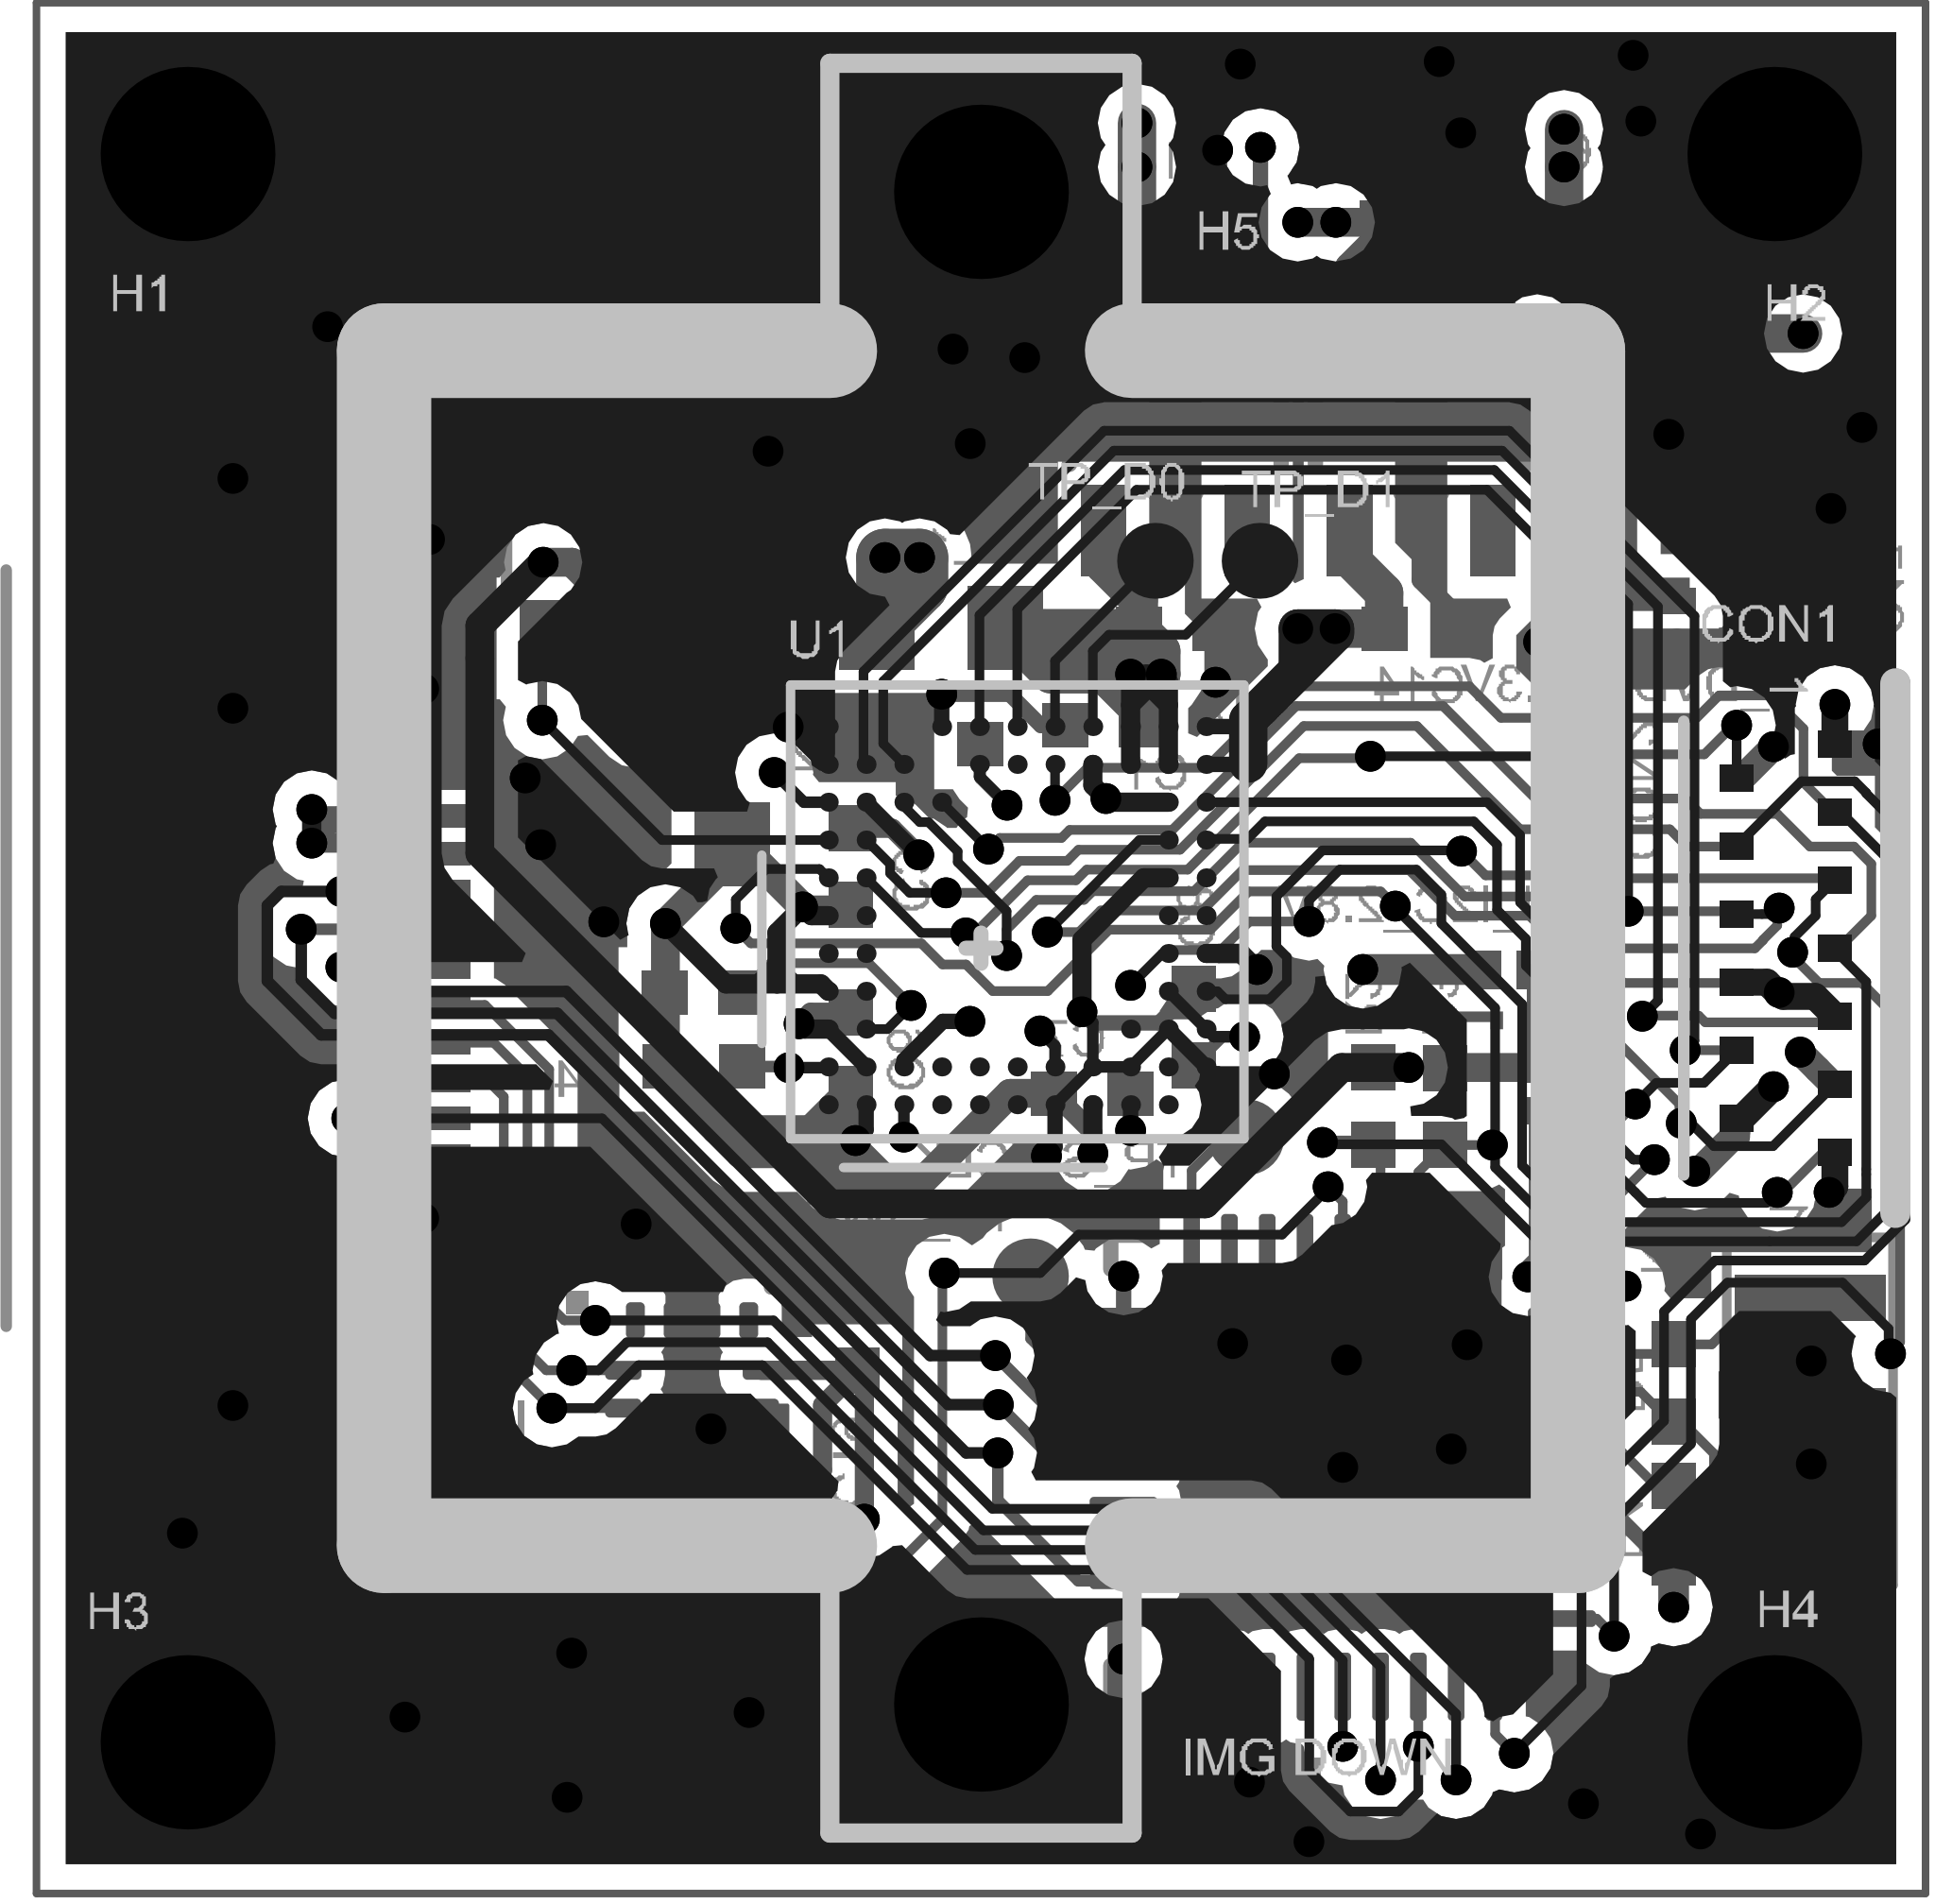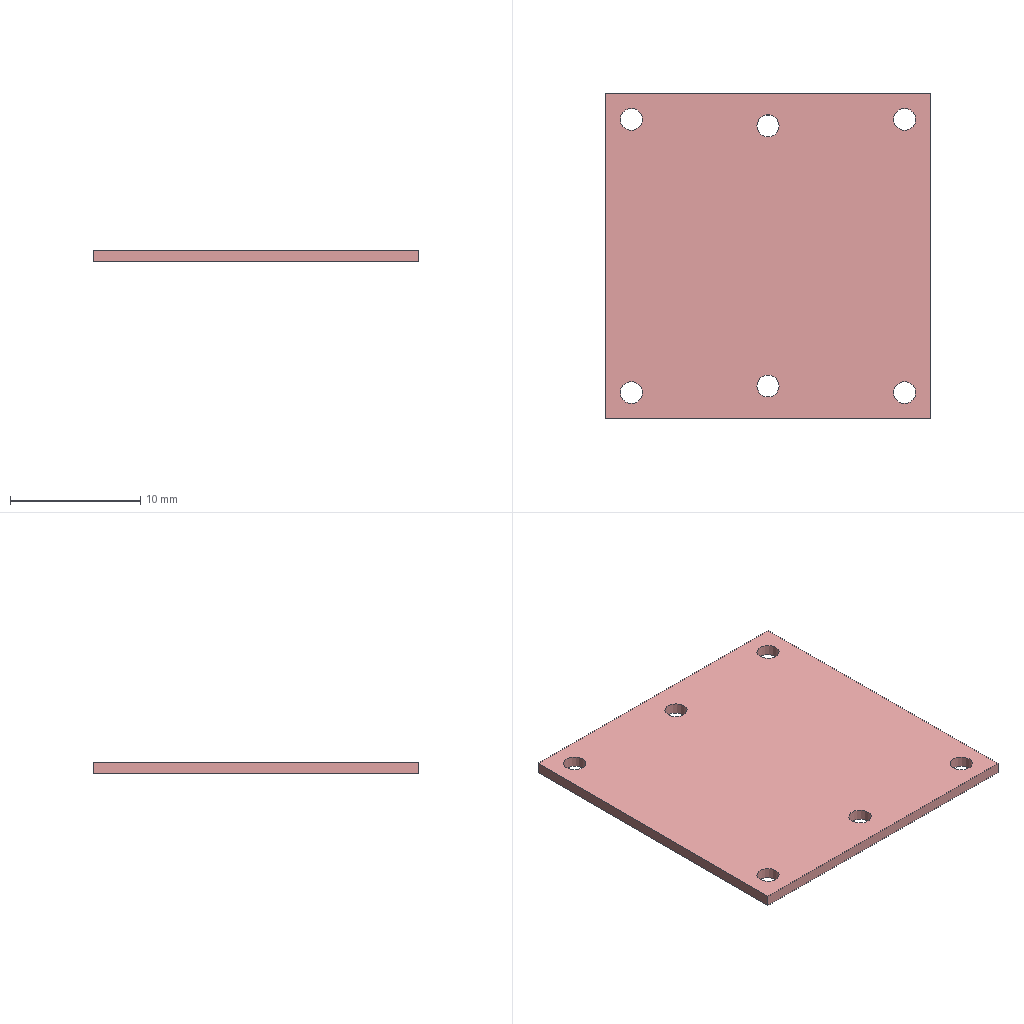Circuit board layout | Altium Designer | box 25 x 25 x 0.9 mm
Layer stack:
# Altium Designer layer stack of  (unit mm; dielectric type: 0 none, 1 core, 2 prepreg, 3 surface material)
index,name,kind,layer,copper_thickness_mm,dielectric_type,dielectric_thickness_mm,dielectric_material,dielectric_constant
0,Top Paste,other,,,,,,
1,Top Overlay,other,,,,,,
2,Top Solder,dielectric,,,3,0.0102,Solder Resist,3.5
3,Component Side,copper,Component Side,0.0356,,,,
4,Dielectric1,dielectric,,,1,0.32,FR-4,4.8
5,Ground Plane,copper,Ground Plane,0.036,,,,
6,Dielectric5,dielectric,,,2,0.127,,4.2
7,Power Plane,copper,Power Plane,0.036,,,,
8,Dielectric6,dielectric,,,1,0.254,,4.2
9,Solder Side,copper,Solder Side,0.0356,,,,
10,Bottom Solder,dielectric,,,3,0.0102,Solder Resist,3.5
11,Bottom Overlay,other,,,,,,
12,Bottom Paste,other,,,,,,
# drill layer pairs: low layer,high layer
drill_pair,Component Side,Solder Side
Part placement:
Designator,Comment,Layer,Footprint,Center-X(mm),Center-Y(mm),Rotation
IC2,QMI8658C,BottomLayer,LGA14_3X2.5,8.676,6.418,270
C19,0.1uF,BottomLayer,RCL_C0402_TI,10.861,7.424,270
X2,4MHz,BottomLayer,XTAL_4.5X2.0,23.47,6.375,90
R5,1M,BottomLayer,RCL_R0402_TI,21.664,6.753,270
R3,2.2K,BottomLayer,RCL_R0402_TI,18.647,10.405,270
R2,2.2K,BottomLayer,RCL_R0402_TI,17.689,10.414,270
R1,1M,BottomLayer,RCL_R0402_TI,7.602,20.302,180
P2R,FPC-12P-0.5-H-NORM,BottomLayer,FPC-12P-0.5-H-NORM,3.862,12.5,90
U1,CMOS sensor,TopLayer,BGA71_5.99X5.84,12.98,12.93,180
C1,1uF,BottomLayer,RCL_C0402_TI,14.124,15.443,180
C2,0.1uF,BottomLayer,RCL_C0402_TI,11.982,15.198,360
C3,0.1uF,BottomLayer,RCL_C0402_TI,10.775,13.577,270
C4,0.1uF,BottomLayer,RCL_C0402_TI,8.832,10.935,180
C5,0.1uF,BottomLayer,RCL_C0402_TI,8.821,11.916,180
C6,0.1uF,BottomLayer,RCL_C0402_TI,10.783,11.144,90
C7,0.1uF,BottomLayer,RCL_C0402_TI,13.97,10.58,360
C8,0.1uF,BottomLayer,RCL_C0402_TI,15.312,11.457,90
C9,10pF,BottomLayer,RCL_C0402_TI,10.463,22.683,90
C10,10pF,BottomLayer,RCL_C0402_TI,4.788,22.693,270
C11,1uF,BottomLayer,RCL_C0402_TI,15.072,22.097,360
C12,1uF,BottomLayer,RCL_C0402_TI,15.097,16.725,360
C13,1uF,BottomLayer,RCL_C0402_TI,18.325,22.097,360
C14,1uF,BottomLayer,RCL_C0402_TI,18.343,16.725,360
C15,0.1uF,BottomLayer,RCL_C0402_TI,9.682,17.856,90
C16,1uF,BottomLayer,RCL_C0402_TI,20.724,22.097,360
C17,1uF,BottomLayer,RCL_C0402_TI,23.75,17.086,90
C18,0.1uF,BottomLayer,RCL_C0402_TI,14.884,1.473,360
H1,MOUNT-HOLE1.7,TopLayer,MOUNT-HOLE1.7,2,23,0
H2,MOUNT-HOLE1.7,TopLayer,MOUNT-HOLE1.7,23,23,0
H3,MOUNT-HOLE1.7,TopLayer,MOUNT-HOLE1.7,2,2,0
H4,MOUNT-HOLE1.7,TopLayer,MOUNT-HOLE1.7,23,2,0
IC1,GD32F103TBU6 36pin QFN,BottomLayer,GD32_QFN36,17.288,5.635,180
L1,470R L,BottomLayer,RCL_L0603,11.966,16.729,360
L2,470R L,BottomLayer,RCL_L0603,8.358,13.868,360
R4,2.2K,BottomLayer,RCL_R0402_TI,21.663,4.886,270
TP_D0,,TopLayer,TP-1,14.802,17.621,270
TP_D1,,TopLayer,TP-1,16.186,17.621,270
U2,NL27WZU04DTT,BottomLayer,SOT23-6,7.644,17.845,360
U3,ME6219SMD-2.8V,BottomLayer,SOT23-5,15.072,19.327,360
U4,ME6219SMD-1.5V,BottomLayer,SOT23-5,18.326,19.327,360
U5,ME6211,BottomLayer,SOT23-5,21.61,19.327,360
X1,24M/9pF,BottomLayer,EPSON-TSX3225,7.599,22.683,90
H5,MOUNT-LENS,TopLayer,MOUNT-LENS-M12-1.6,12.5,12.5,90
CON1,13P-0.5-36AWG,TopLayer,13P-0.5-36AWG,23.15,12.5,90
CON2,13P-0.5-36AWG,BottomLayer,13P-0.5-36AWG,23.15,12.5,270
J_I2C_2.8V,JUMPER_2P_MIN,BottomLayer,JUMPER_2P_MIN,19.482,12.217,180
J_I2C_3.3V,JUMPER_2P_MIN,BottomLayer,JUMPER_2P_MIN,19.94,10.63,270
TP_SWCLK,,BottomLayer,TP-1,16,10,90
TP_SWDIO,,BottomLayer,TP-1,13.15,8.16,90
J_DVDD_3.3V,JUMPER_2P_MIN,BottomLayer,JUMPER_2P_MIN,21.71,16.81,270
Pad and via stacks:
# Altium Designer via and pad stacks of  (unit mm). Each distinct definition once, with the count of objects using it.
# via: kind,start_layer,end_layer,hole_mm,diameter_mm,mode(0 simple;1 top-mid-bottom;2 full stack),diameter_per_layer,count,example_net
# pad: kind,layer,hole_mm,hole_type(0 round;1 square;2 slot),plating,top_size,top_shape(1 round;2 rect;3 octagon;9 rounded rect),mid_size,bottom_size,mode,footprint,size_per_layer,count,example
pad,Multi-Layer,1.7,0,plated,2.3x2.3,1,2.3x2.3,2.3x2.3,0,MOUNT-HOLE1.7,,4,H3.MOUNT
pad,Multi-Layer,1.7,0,plated,2.3x2.3,1,2.3x2.3,2.3x2.3,0,MOUNT-LENS-M12-1.6,,2,H5.MOUNT
pad,Solder Side,0,0,plated,0.35x0.5,2,0.35x0.5,0.35x0.5,0,JUMPER_2P_MIN,,6,J_I2C_3.3V.1
pad,Solder Side,0,0,plated,1x1,1,1x1,1x1,0,TP-1,,2,TP_SWDIO.1
pad,Solder Side,0,0,plated,0.35x0.45,2,0.35x0.45,0.35x0.45,0,13P-0.5-36AWG,,13,CON2.P$8
pad,Solder Side,0,0,plated,0.6096x0.5842,2,0.6096x0.5842,0.6096x0.5842,0,RCL_C0402_TI,,38,C19.1
pad,Solder Side,0,0,plated,0.6096x0.5842,2,0.6096x0.5842,0.6096x0.5842,0,RCL_R0402_TI,,10,R5.2
pad,Solder Side,0,0,plated,0.6x1.2,2,0.6x1.2,0.6x1.2,0,SOT23-5,,15,U4.1
pad,Solder Side,0,0,plated,1x1.1,2,1x1.1,1x1.1,0,RCL_L0603,,4,L1.2
pad,Solder Side,0,0,plated,1.15x1.4,2,1.15x1.4,1.15x1.4,0,EPSON-TSX3225,,4,X1.3
pad,Solder Side,0,0,plated,0.6x1,2,0.6x1,0.6x1,0,SOT23-6,,6,U2.1
pad,Solder Side,0,0,plated,0.9x0.22,9,0.9x0.22,0.9x0.22,0,GD32_QFN36,,36,IC1.31
pad,Solder Side,0,0,plated,3x3,2,3x3,3x3,0,GD32_QFN36,,1,IC1.5
pad,Solder Side,0,0,plated,0.3x1.25,2,0.3x1.25,0.3x1.25,0,FPC-12P-0.5-H-NORM,,12,P2R.P$11
pad,Solder Side,0,0,plated,1.8x2.2,2,1.8x2.2,1.8x2.2,0,FPC-12P-0.5-H-NORM,,2,P2R.M
pad,Solder Side,0,0,plated,0.6x2,2,0.6x2,0.6x2,0,XTAL_4.5X2.0,,3,X2.3
pad,Solder Side,0,0,plated,0.48x0.25,9,0.48x0.25,0.48x0.25,0,LGA14_3X2.5,,14,IC2.7
pad,Component Side,0,0,plated,0.35x0.45,2,0.35x0.45,0.35x0.45,0,13P-0.5-36AWG,,13,CON1.P$8
pad,Component Side,0,0,plated,1x1,1,1x1,1x1,0,TP-1,,2,TP_D0.1
pad,Component Side,0,0,plated,0.25x0.25,1,0.25x0.25,0.25x0.25,0,BGA71_5.99X5.84,,71,U1.I9
via,Component Side,Solder Side,0.2032,0.4064,0,,152,MCU_RX
Copper pours:
name,layer,net,type(0 solid;1 hatched;2 none)
Top Layer-No Net,Component Side,DGND,0
Bottom Layer-No Net,Solder Side,DVDD_3.3V,0
Bottom Layer-No Net,Solder Side,NetJ_DVDD_3.3V_1,0
Top Layer-No Net,Solder Side,DGND,0
Design rules, without the lines most boards share:
# Altium Designer design rules of  (exported by Altium Designer, unit mm)
# columns: name | kind | enabled | priority | scope1 | scope2 | descriptor | typed fields (field=value)
Clearance_1 | 0 | enabled | 1 | InPolygon | All | Clearance Constraint (Gap=12mil) (InPolygon),(All) | gap=0.3048
Clearance | 0 | enabled | 2 | All | All | Clearance Constraint (Gap=5mil) (All),(All) | gap=0.127
PlaneConnect | 6 | enabled | 1 | All | All | Power Plane Connect Rule(Direct Connect )(Expansion=20mil) (Conductor Width=10mil) (Air Gap=10mil) (Entries=4) (All) | relief_conductor_width=0.254 relief_entries=4 relief_expansion=0.508
PlaneClearance | 12 | enabled | 1 | All | All | Power Plane Clearance (Clearance =6mil) (All) | clearance=0.1524
PolygonConnect | 20 | enabled | 1 | All | All | Polygon Connect Rule(Direct Connect )(Conductor Width=10mil) (Relief Angle=90 Angle) (Entries=4) (Air Gap Width=10mil) (All),(All) | connect_style(0=relief,1=direct,2=none)=1 relief_conductor_width=0.254 relief_entries=4
Width | 2 | enabled | 1 | All | All | Width Constraint (Min=5mil) (Max=200mil) (Preferred=5mil) (All) |
RoutingPriority | 8 | disabled | 1 | All | All | TRoutingPriorityRule(Priority=0) (Disabled)(All) |
RoutingLayers | 9 | disabled | 1 | All | All | Routing Layers(Disabled)(All) |
RoutingCorners | 10 | disabled | 1 | All | All | Routing Corners (Style=45-Degree) (Min Setback=100mil) (Max Setback=100mil) (Disabled)(All) |
RoutingVias | 11 | enabled | 1 | All | All | Routing Via (MinHoleWidth=8mil) (MaxHoleWidth=8mil) (PreferredHoleWidth=8mil) (MinWidth=16mil) (MaxWidth=16mil) (PreferedWidth=16mil) (All) | via_min_hole=0.2032 via_max_hole=0.2032 via_preferred_diameter=0.4064 via_preferred_hole=0.2032
PasteMaskExpansion | 14 | disabled | 1 | All | All | Paste Mask Expansion (Expansion =0mil) (Disabled)(All) | expansion=0
SolderMaskExpansion | 13 | disabled | 1 | All | All | Solder Mask Expansion (Expansion =4mil) (Disabled)(All) | expansion=0.1016
RoutingTopology | 7 | disabled | 1 | All | All | Routing Topology Rule(Topology=Shortest) (Disabled)(All) |
FabricationTestPointUsage | 44 | disabled | 1 | All | All | Fabrication Testpoint Usage (Valid =One Required, Allow multiple per net=No) (Disabled)(All) |
FabricationTestpoint | 43 | disabled | 1 | All | All | Fabrication Testpoint Style (Under Component=Yes) (Disabled)(All) |
AssemblyTestPointUsage | 58 | disabled | 1 | All | All | Assembly Testpoint Usage (Valid =One Required, Allow multiple per net=No) (Disabled)(All) |
AssemblyTestpoint | 57 | disabled | 1 | All | All | Assembly Testpoint Style (Under Component=Yes) (Disabled)(All) |
ComponentClearance | 24 | disabled | 1 | All | All | Component Clearance Constraint ( Horizontal Gap = 10mil, Vertical Gap = 10mil ) (Disabled)(All),(All)  | gap=0.254
Height | 50 | disabled | 1 | All | All | Height Constraint (Min=0mil) (Max=1000mil) (Prefered=500mil) (Disabled)(All) | min_height=0 max_height=25.4
LayerPairs | 48 | disabled | 1 | All | All | Pads and Vias to follow the Drill pairs settings |
HoleSize | 42 | disabled | 1 | All | All | Hole Size Constraint (Min=1mil) (Max=500mil) (Disabled)(All) |
Fanout_Default | 49 | disabled | 5 | All | All | Fanout Control Rule ( (Disabled)(All) ) |
Fanout_Small | 49 | disabled | 4 | (CompPinCount < 5) | All | Fanout Control Rule ( (Disabled)((CompPinCount < 5)) ) |
Fanout_SOIC | 49 | disabled | 3 | IsSOIC | All | Fanout Control Rule ( (Disabled)(IsSOIC) ) |
Fanout_LCC | 49 | disabled | 2 | IsLCC | All | Fanout Control Rule ( (Disabled)(IsLCC) ) |
Fanout_BGA | 49 | disabled | 1 | IsBGA | All | Fanout Control Rule ( (Disabled)(IsBGA) ) |
DiffPairsRouting | 51 | disabled | 1 | All | All | Differential Pairs Uncoupled Length using the Gap Constraints (Min=10mil) (Max=10mil) (Prefered=10mil)  and Width Constraints (Min=15mil) (Max=15mil) (Prefered=15mil) (Disabled)(All) |
HoleToHoleClearance | 52 | disabled | 1 | All | All | Hole To Hole Clearance (Gap=0mil) (Disabled)(All),(All) | gap=0
MinimumSolderMaskSliver | 53 | disabled | 1 | All | All | Minimum Solder Mask Sliver (Gap=0mil) (Disabled)(All),(All) |
SilkToSolderMaskClearance | 54 | disabled | 1 | IsPad | All | Silk To Solder Mask (Clearance=0mil) (Disabled)(IsPad),(All) |
SilkToSilkClearance | 55 | disabled | 1 | All | All | Silk to Silk (Clearance=0mil) (Disabled)(All),(All) |
NetAntennae | 56 | disabled | 1 | All | All | Net Antennae (Tolerance=0mil) (Disabled)(All) |
Classes set for this board:
# Altium Designer classes of  (member kind: 0 net, 1 component, 2 from-to, 3 pad, 4 layer, 5 differential pair, 6 design channel, 7 polygon, 8 structure, 9 xSignal)
# columns: class name | member kind | superclass | members
CM1v07 | 1 | no | U1; P2R; C7; C16; C17; C18; IC1; R4; TP_D0; TP_D1; U5; H1; H2; H3; H4; H5; R2; R3; C1; C2; C3; C4; C5; C6; C8; C9; C10; C11; C12; C13; C14; C15; L1; L2; R1; U2; U3; U4; X1; R5; X2; C19; IC2; CON1; CON2; TP_SWCLK; TP_SWDIO; J_DVDD_3.3V; J_I2C_2.8V; J_I2C_3.3V;